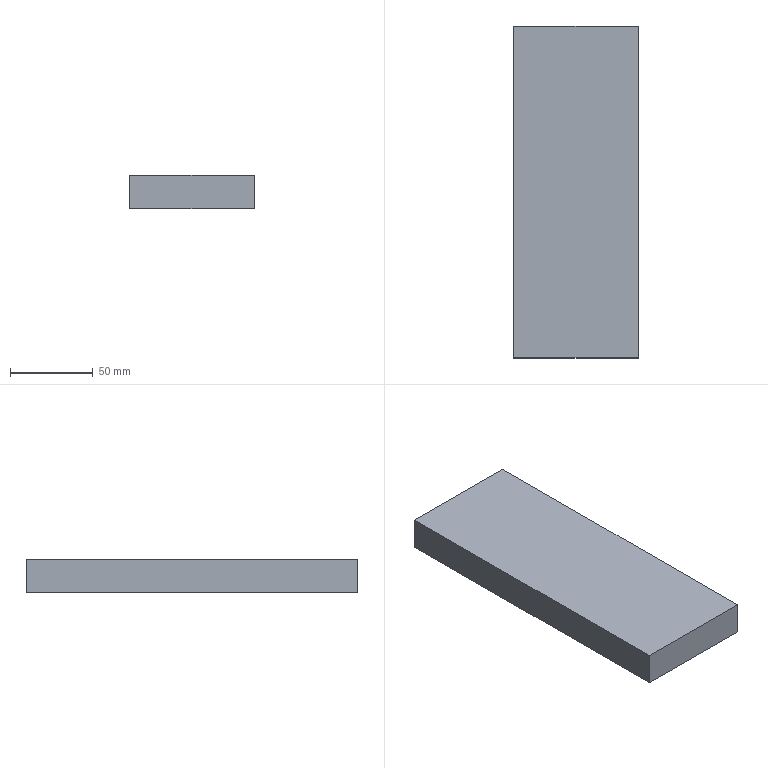Part | NX | features solid 2 | 1 solid | 6 faces | box 75 x 200 x 20 mm | volume 300000 mm3 | plane 6
STEP:
#1=CARTESIAN_POINT('',(457.5,475.,-375.));
#2=VERTEX_POINT('',#1);
#3=CARTESIAN_POINT('',(457.5,475.,-355.));
#4=VERTEX_POINT('',#3);
#5=CARTESIAN_POINT('',(457.5,475.,-365.));
#6=DIRECTION('',(0.,0.,1.));
#7=VECTOR('',#6,1000.);
#8=LINE('',#5,#7);
#9=EDGE_CURVE('',#2,#4,#8,.T.);
#10=ORIENTED_EDGE('',*,*,#9,.T.);
#11=CARTESIAN_POINT('',(382.5,475.,-355.));
#12=VERTEX_POINT('',#11);
#13=CARTESIAN_POINT('',(345.,475.,-355.));
#14=DIRECTION('',(1.,0.,0.));
#15=VECTOR('',#14,1000.);
#16=LINE('',#13,#15);
#17=EDGE_CURVE('',#12,#4,#16,.T.);
#18=ORIENTED_EDGE('',*,*,#17,.F.);
#19=CARTESIAN_POINT('',(382.5,475.,-375.));
#20=VERTEX_POINT('',#19);
#21=CARTESIAN_POINT('',(382.5,475.,-365.));
#22=DIRECTION('',(0.,0.,1.));
#23=VECTOR('',#22,1000.);
#24=LINE('',#21,#23);
#25=EDGE_CURVE('',#20,#12,#24,.T.);
#26=ORIENTED_EDGE('',*,*,#25,.F.);
#27=CARTESIAN_POINT('',(345.,475.,-375.));
#28=DIRECTION('',(1.,0.,0.));
#29=VECTOR('',#28,1000.);
#30=LINE('',#27,#29);
#31=EDGE_CURVE('',#20,#2,#30,.T.);
#32=ORIENTED_EDGE('',*,*,#31,.T.);
#33=EDGE_LOOP('',(#10,#18,#26,#32));
#34=FACE_BOUND('',#33,.T.);
#35=CARTESIAN_POINT('',(345.,475.,-375.));
#36=DIRECTION('',(0.,-1.,0.));
#37=DIRECTION('',(0.,0.,-1.));
#38=AXIS2_PLACEMENT_3D('',#35,#36,#37);
#39=PLANE('',#38);
#40=ADVANCED_FACE('',(#34),#39,.T.);
#41=CARTESIAN_POINT('',(457.5,675.,-375.));
#42=VERTEX_POINT('',#41);
#43=CARTESIAN_POINT('',(457.5,628.851,-375.));
#44=DIRECTION('',(0.,-1.,0.));
#45=VECTOR('',#44,1000.);
#46=LINE('',#43,#45);
#47=EDGE_CURVE('',#42,#2,#46,.T.);
#48=ORIENTED_EDGE('',*,*,#47,.T.);
#49=ORIENTED_EDGE('',*,*,#31,.F.);
#50=CARTESIAN_POINT('',(382.5,675.,-375.));
#51=VERTEX_POINT('',#50);
#52=CARTESIAN_POINT('',(382.5,628.851,-375.));
#53=DIRECTION('',(0.,-1.,0.));
#54=VECTOR('',#53,1000.);
#55=LINE('',#52,#54);
#56=EDGE_CURVE('',#51,#20,#55,.T.);
#57=ORIENTED_EDGE('',*,*,#56,.F.);
#58=CARTESIAN_POINT('',(345.,675.,-375.));
#59=DIRECTION('',(1.,0.,0.));
#60=VECTOR('',#59,1000.);
#61=LINE('',#58,#60);
#62=EDGE_CURVE('',#51,#42,#61,.T.);
#63=ORIENTED_EDGE('',*,*,#62,.T.);
#64=EDGE_LOOP('',(#48,#49,#57,#63));
#65=FACE_BOUND('',#64,.T.);
#66=CARTESIAN_POINT('',(345.,675.,-375.));
#67=DIRECTION('',(0.,0.,-1.));
#68=DIRECTION('',(1.,0.,0.));
#69=AXIS2_PLACEMENT_3D('',#66,#67,#68);
#70=PLANE('',#69);
#71=ADVANCED_FACE('',(#65),#70,.T.);
#72=CARTESIAN_POINT('',(457.5,675.,-355.));
#73=VERTEX_POINT('',#72);
#74=CARTESIAN_POINT('',(457.5,675.,-365.));
#75=DIRECTION('',(0.,0.,1.));
#76=VECTOR('',#75,1000.);
#77=LINE('',#74,#76);
#78=EDGE_CURVE('',#42,#73,#77,.T.);
#79=ORIENTED_EDGE('',*,*,#78,.F.);
#80=ORIENTED_EDGE('',*,*,#62,.F.);
#81=CARTESIAN_POINT('',(382.5,675.,-355.));
#82=VERTEX_POINT('',#81);
#83=CARTESIAN_POINT('',(382.5,675.,-365.));
#84=DIRECTION('',(0.,0.,1.));
#85=VECTOR('',#84,1000.);
#86=LINE('',#83,#85);
#87=EDGE_CURVE('',#51,#82,#86,.T.);
#88=ORIENTED_EDGE('',*,*,#87,.T.);
#89=CARTESIAN_POINT('',(345.,675.,-355.));
#90=DIRECTION('',(1.,0.,0.));
#91=VECTOR('',#90,1000.);
#92=LINE('',#89,#91);
#93=EDGE_CURVE('',#82,#73,#92,.T.);
#94=ORIENTED_EDGE('',*,*,#93,.T.);
#95=EDGE_LOOP('',(#79,#80,#88,#94));
#96=FACE_BOUND('',#95,.T.);
#97=CARTESIAN_POINT('',(345.,675.,-375.));
#98=DIRECTION('',(0.,-1.,0.));
#99=DIRECTION('',(0.,0.,-1.));
#100=AXIS2_PLACEMENT_3D('',#97,#98,#99);
#101=PLANE('',#100);
#102=ADVANCED_FACE('',(#96),#101,.F.);
#103=CARTESIAN_POINT('',(457.5,628.851,-355.));
#104=DIRECTION('',(0.,-1.,0.));
#105=VECTOR('',#104,1000.);
#106=LINE('',#103,#105);
#107=EDGE_CURVE('',#73,#4,#106,.T.);
#108=ORIENTED_EDGE('',*,*,#107,.F.);
#109=ORIENTED_EDGE('',*,*,#93,.F.);
#110=CARTESIAN_POINT('',(382.5,628.851,-355.));
#111=DIRECTION('',(0.,-1.,0.));
#112=VECTOR('',#111,1000.);
#113=LINE('',#110,#112);
#114=EDGE_CURVE('',#82,#12,#113,.T.);
#115=ORIENTED_EDGE('',*,*,#114,.T.);
#116=ORIENTED_EDGE('',*,*,#17,.T.);
#117=EDGE_LOOP('',(#108,#109,#115,#116));
#118=FACE_BOUND('',#117,.T.);
#119=CARTESIAN_POINT('',(345.,690.404,-355.));
#120=DIRECTION('',(0.,0.,-1.));
#121=DIRECTION('',(1.,0.,0.));
#122=AXIS2_PLACEMENT_3D('',#119,#120,#121);
#123=PLANE('',#122);
#124=ADVANCED_FACE('',(#118),#123,.F.);
#125=ORIENTED_EDGE('',*,*,#25,.T.);
#126=ORIENTED_EDGE('',*,*,#114,.F.);
#127=ORIENTED_EDGE('',*,*,#87,.F.);
#128=ORIENTED_EDGE('',*,*,#56,.T.);
#129=EDGE_LOOP('',(#125,#126,#127,#128));
#130=FACE_BOUND('',#129,.T.);
#131=CARTESIAN_POINT('',(382.5,628.851,-365.));
#132=DIRECTION('',(-1.,0.,0.));
#133=DIRECTION('',(0.,0.,-1.));
#134=AXIS2_PLACEMENT_3D('',#131,#132,#133);
#135=PLANE('',#134);
#136=ADVANCED_FACE('',(#130),#135,.T.);
#137=ORIENTED_EDGE('',*,*,#9,.F.);
#138=ORIENTED_EDGE('',*,*,#47,.F.);
#139=ORIENTED_EDGE('',*,*,#78,.T.);
#140=ORIENTED_EDGE('',*,*,#107,.T.);
#141=EDGE_LOOP('',(#137,#138,#139,#140));
#142=FACE_BOUND('',#141,.T.);
#143=CARTESIAN_POINT('',(457.5,628.851,-365.));
#144=DIRECTION('',(-1.,0.,0.));
#145=DIRECTION('',(0.,0.,-1.));
#146=AXIS2_PLACEMENT_3D('',#143,#144,#145);
#147=PLANE('',#146);
#148=ADVANCED_FACE('',(#142),#147,.F.);
#149=CLOSED_SHELL('',(#40,#71,#102,#124,#136,#148));
#150=MANIFOLD_SOLID_BREP('',#149);
#151=(LENGTH_UNIT()NAMED_UNIT(*)SI_UNIT(.MILLI.,.METRE.));
#152=UNCERTAINTY_MEASURE_WITH_UNIT(LENGTH_MEASURE(0.00001),#151,'','');
#153=(NAMED_UNIT(*)PLANE_ANGLE_UNIT()SI_UNIT($,.RADIAN.));
#154=(NAMED_UNIT(*)SI_UNIT($,.STERADIAN.)SOLID_ANGLE_UNIT());
#155=(GEOMETRIC_REPRESENTATION_CONTEXT(3)GLOBAL_UNCERTAINTY_ASSIGNED_CONTEXT((#152))GLOBAL_UNIT_ASSIGNED_CONTEXT((#151,#153,#154))REPRESENTATION_CONTEXT('',''));
#156=ADVANCED_BREP_SHAPE_REPRESENTATION('',(#150),#155);